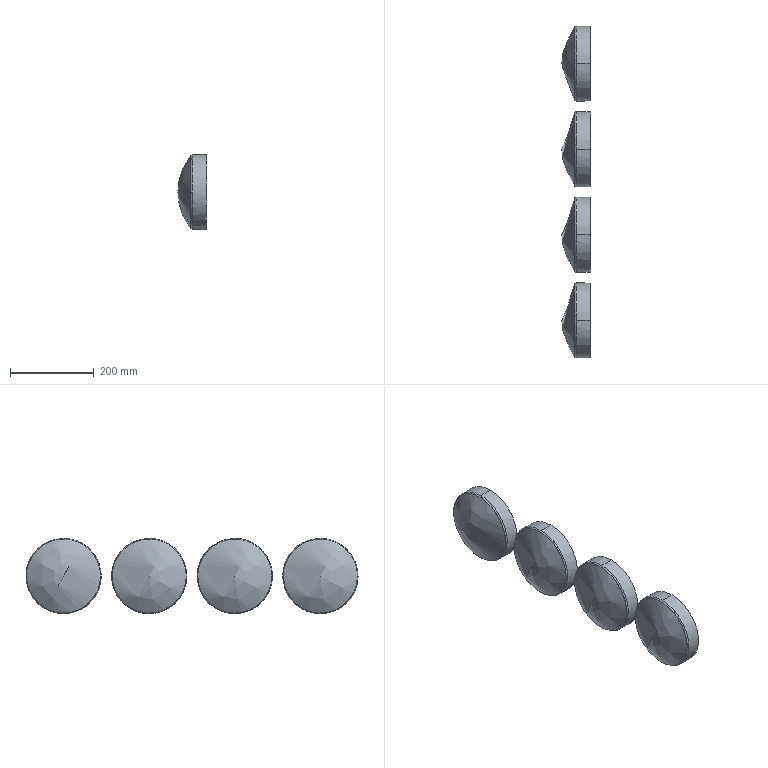Part | STEP file | Imported10 | 2 solids | 37 faces | box 68 x 795 x 180 mm | volume 2663034 mm3 | spline 25 | cylinder 8 | plane 4 | commonest cylinder face diameters 180 x8